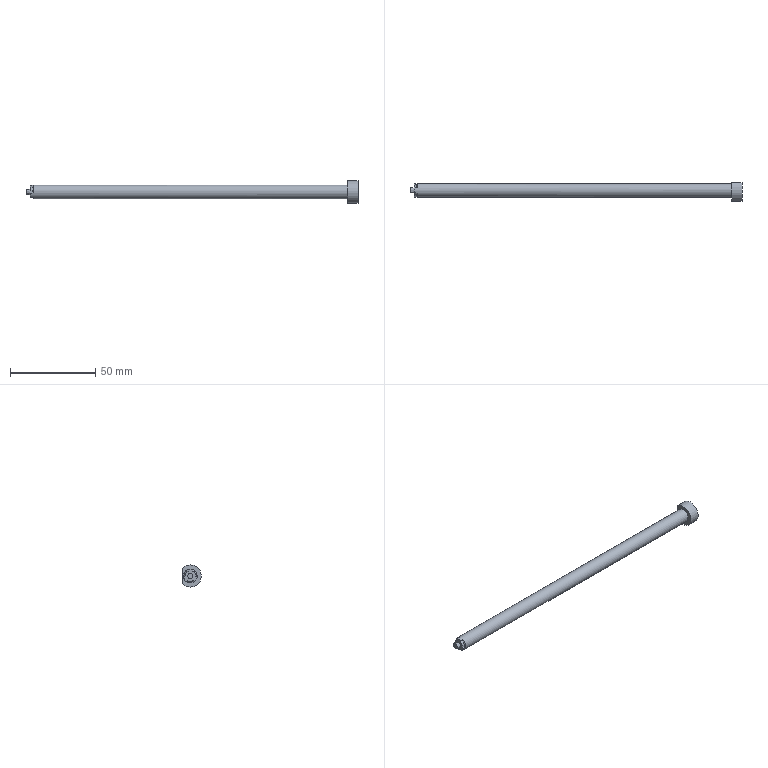Part | STEP file | solid 146 | 1 solid | 23 faces | box 195.123 x 11 x 13 mm | volume 10096 mm3 | spline 12 | plane 9 | cylinder 2 | commonest cylinder face diameters 8 x1 13 x1